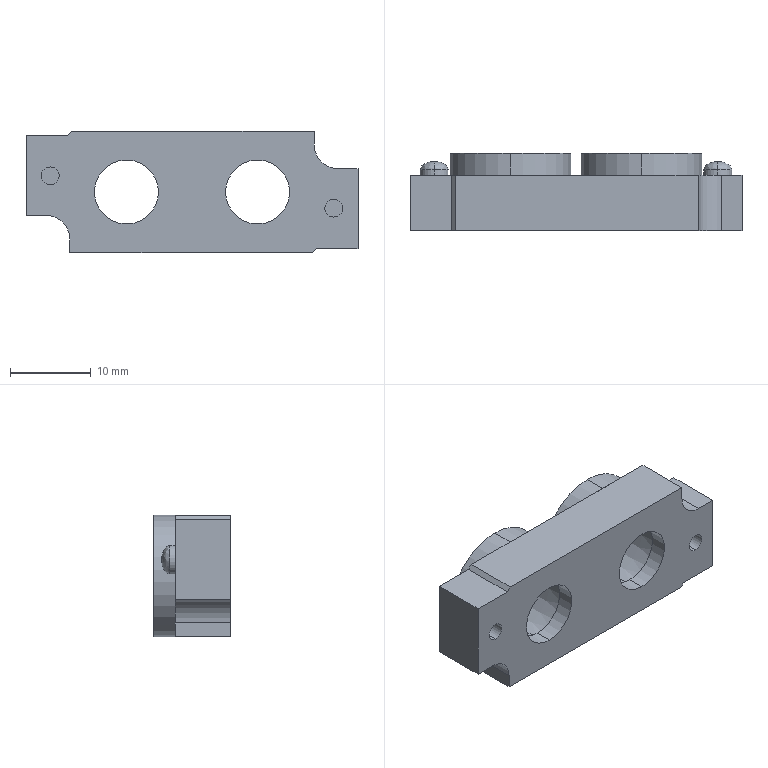Part | STEP file | 11-sy5120-5gz-01_sy5000-6-1-V2.0-V2.011_01 | 1 solid | 48 faces | box 41 x 9.5 x 15 mm | volume 3507 mm3 | plane 22 | cylinder 18 | spline 4 | cone 4 | commonest cylinder face diameters 2.2 x4 3.5 x4 7.9 x4 15 x4 5.8 x2
STEP:
#1=CARTESIAN_POINT('',(-17.5,8.5,2.));
#2=VERTEX_POINT('',#1);
#3=CARTESIAN_POINT('',(-17.5,7.5,3.75));
#4=VERTEX_POINT('',#3);
#5=CARTESIAN_POINT('',(-17.5,8.5,2.));
#6=CARTESIAN_POINT('',(-17.5,8.5,3.025));
#7=CARTESIAN_POINT('',(-17.5,8.086,3.75));
#8=CARTESIAN_POINT('',(-17.5,7.5,3.75));
#9=(BOUNDED_CURVE()B_SPLINE_CURVE(3,(#5,#6,#7,#8),.UNSPECIFIED.,.F.,.F.)B_SPLINE_CURVE_WITH_KNOTS((4,4),(4.712,6.283),.UNSPECIFIED.)CURVE()GEOMETRIC_REPRESENTATION_ITEM()RATIONAL_B_SPLINE_CURVE((1.,0.8047,0.8047,1.))REPRESENTATION_ITEM(''));
#10=EDGE_CURVE('',#2,#4,#9,.T.);
#11=ORIENTED_EDGE('',*,*,#10,.F.);
#12=CARTESIAN_POINT('',(-17.5,7.5,0.25));
#13=VERTEX_POINT('',#12);
#14=CARTESIAN_POINT('',(-17.5,8.5,2.));
#15=CARTESIAN_POINT('',(-17.5,8.5,0.9749));
#16=CARTESIAN_POINT('',(-17.5,8.086,0.25));
#17=CARTESIAN_POINT('',(-17.5,7.5,0.25));
#18=(BOUNDED_CURVE()B_SPLINE_CURVE(3,(#14,#15,#16,#17),.UNSPECIFIED.,.F.,.F.)B_SPLINE_CURVE_WITH_KNOTS((4,4),(4.712,6.283),.UNSPECIFIED.)CURVE()GEOMETRIC_REPRESENTATION_ITEM()RATIONAL_B_SPLINE_CURVE((1.,0.8047,0.8047,1.))REPRESENTATION_ITEM(''));
#19=EDGE_CURVE('',#2,#13,#18,.T.);
#20=ORIENTED_EDGE('',*,*,#19,.T.);
#21=CARTESIAN_POINT('',(-17.5,7.5,2.));
#22=DIRECTION('',(0.,1.,0.));
#23=DIRECTION('',(0.,0.,1.));
#24=AXIS2_PLACEMENT_3D('',#21,#22,#23);
#25=CIRCLE('',#24,1.75);
#26=EDGE_CURVE('',#13,#4,#25,.T.);
#27=ORIENTED_EDGE('',*,*,#26,.T.);
#28=EDGE_LOOP('',(#11,#20,#27));
#29=FACE_OUTER_BOUND('',#28,.T.);
#30=CARTESIAN_POINT('',(-17.5,8.5,2.));
#31=CARTESIAN_POINT('',(-17.5,8.5,2.));
#32=CARTESIAN_POINT('',(-17.5,8.5,2.));
#33=CARTESIAN_POINT('',(-17.5,8.5,2.));
#34=CARTESIAN_POINT('',(-17.5,8.5,0.9749));
#35=CARTESIAN_POINT('',(-19.55,8.5,0.9749));
#36=CARTESIAN_POINT('',(-19.55,8.5,3.025));
#37=CARTESIAN_POINT('',(-17.5,8.5,3.025));
#38=CARTESIAN_POINT('',(-17.5,8.086,0.25));
#39=CARTESIAN_POINT('',(-21.,8.086,0.25));
#40=CARTESIAN_POINT('',(-21.,8.086,3.75));
#41=CARTESIAN_POINT('',(-17.5,8.086,3.75));
#42=CARTESIAN_POINT('',(-17.5,7.5,0.25));
#43=CARTESIAN_POINT('',(-21.,7.5,0.25));
#44=CARTESIAN_POINT('',(-21.,7.5,3.75));
#45=CARTESIAN_POINT('',(-17.5,7.5,3.75));
#46=(BOUNDED_SURFACE()B_SPLINE_SURFACE(3,3,((#30,#31,#32,#33),(#34,#35,#36,#37),(#38,#39,#40,#41),(#42,#43,#44,#45)),.UNSPECIFIED.,.F.,.F.,.F.)B_SPLINE_SURFACE_WITH_KNOTS((4,4),(4,4),(0.,1.),(0.,1.),.UNSPECIFIED.)GEOMETRIC_REPRESENTATION_ITEM()RATIONAL_B_SPLINE_SURFACE(((1.,0.3333,0.3333,1.),(0.8047,0.2682,0.2682,0.8047),(0.8047,0.2682,0.2682,0.8047),(1.,0.3333,0.3333,1.)))REPRESENTATION_ITEM('')SURFACE());
#47=ADVANCED_FACE('',(#29),#46,.T.);
#48=CARTESIAN_POINT('',(17.5,8.5,-2.));
#49=VERTEX_POINT('',#48);
#50=CARTESIAN_POINT('',(17.5,7.5,-0.25));
#51=VERTEX_POINT('',#50);
#52=CARTESIAN_POINT('',(17.5,8.5,-2.));
#53=CARTESIAN_POINT('',(17.5,8.5,-0.9749));
#54=CARTESIAN_POINT('',(17.5,8.086,-0.25));
#55=CARTESIAN_POINT('',(17.5,7.5,-0.25));
#56=(BOUNDED_CURVE()B_SPLINE_CURVE(3,(#52,#53,#54,#55),.UNSPECIFIED.,.F.,.F.)B_SPLINE_CURVE_WITH_KNOTS((4,4),(4.712,6.283),.UNSPECIFIED.)CURVE()GEOMETRIC_REPRESENTATION_ITEM()RATIONAL_B_SPLINE_CURVE((1.,0.8047,0.8047,1.))REPRESENTATION_ITEM(''));
#57=EDGE_CURVE('',#49,#51,#56,.T.);
#58=ORIENTED_EDGE('',*,*,#57,.F.);
#59=CARTESIAN_POINT('',(17.5,7.5,-3.75));
#60=VERTEX_POINT('',#59);
#61=CARTESIAN_POINT('',(17.5,8.5,-2.));
#62=CARTESIAN_POINT('',(17.5,8.5,-3.025));
#63=CARTESIAN_POINT('',(17.5,8.086,-3.75));
#64=CARTESIAN_POINT('',(17.5,7.5,-3.75));
#65=(BOUNDED_CURVE()B_SPLINE_CURVE(3,(#61,#62,#63,#64),.UNSPECIFIED.,.F.,.F.)B_SPLINE_CURVE_WITH_KNOTS((4,4),(4.712,6.283),.UNSPECIFIED.)CURVE()GEOMETRIC_REPRESENTATION_ITEM()RATIONAL_B_SPLINE_CURVE((1.,0.8047,0.8047,1.))REPRESENTATION_ITEM(''));
#66=EDGE_CURVE('',#49,#60,#65,.T.);
#67=ORIENTED_EDGE('',*,*,#66,.T.);
#68=CARTESIAN_POINT('',(17.5,7.5,-2.));
#69=DIRECTION('',(0.,1.,0.));
#70=DIRECTION('',(0.,0.,1.));
#71=AXIS2_PLACEMENT_3D('',#68,#69,#70);
#72=CIRCLE('',#71,1.75);
#73=EDGE_CURVE('',#60,#51,#72,.T.);
#74=ORIENTED_EDGE('',*,*,#73,.T.);
#75=EDGE_LOOP('',(#58,#67,#74));
#76=FACE_OUTER_BOUND('',#75,.T.);
#77=CARTESIAN_POINT('',(17.5,8.5,-2.));
#78=CARTESIAN_POINT('',(17.5,8.5,-2.));
#79=CARTESIAN_POINT('',(17.5,8.5,-2.));
#80=CARTESIAN_POINT('',(17.5,8.5,-2.));
#81=CARTESIAN_POINT('',(17.5,8.5,-3.025));
#82=CARTESIAN_POINT('',(15.45,8.5,-3.025));
#83=CARTESIAN_POINT('',(15.45,8.5,-0.9749));
#84=CARTESIAN_POINT('',(17.5,8.5,-0.9749));
#85=CARTESIAN_POINT('',(17.5,8.086,-3.75));
#86=CARTESIAN_POINT('',(14.,8.086,-3.75));
#87=CARTESIAN_POINT('',(14.,8.086,-0.25));
#88=CARTESIAN_POINT('',(17.5,8.086,-0.25));
#89=CARTESIAN_POINT('',(17.5,7.5,-3.75));
#90=CARTESIAN_POINT('',(14.,7.5,-3.75));
#91=CARTESIAN_POINT('',(14.,7.5,-0.25));
#92=CARTESIAN_POINT('',(17.5,7.5,-0.25));
#93=(BOUNDED_SURFACE()B_SPLINE_SURFACE(3,3,((#77,#78,#79,#80),(#81,#82,#83,#84),(#85,#86,#87,#88),(#89,#90,#91,#92)),.UNSPECIFIED.,.F.,.F.,.F.)B_SPLINE_SURFACE_WITH_KNOTS((4,4),(4,4),(0.,1.),(0.,1.),.UNSPECIFIED.)GEOMETRIC_REPRESENTATION_ITEM()RATIONAL_B_SPLINE_SURFACE(((1.,0.3333,0.3333,1.),(0.8047,0.2682,0.2682,0.8047),(0.8047,0.2682,0.2682,0.8047),(1.,0.3333,0.3333,1.)))REPRESENTATION_ITEM('')SURFACE());
#94=ADVANCED_FACE('',(#76),#93,.T.);
#95=CARTESIAN_POINT('',(-8.1,2.1,-4.633));
#96=VERTEX_POINT('',#95);
#97=CARTESIAN_POINT('',(-8.1,2.1,4.633));
#98=VERTEX_POINT('',#97);
#99=CARTESIAN_POINT('',(-8.1,2.1,0.));
#100=DIRECTION('',(0.,1.,0.));
#101=DIRECTION('',(0.,0.,1.));
#102=AXIS2_PLACEMENT_3D('',#99,#100,#101);
#103=CIRCLE('',#102,4.633);
#104=EDGE_CURVE('',#96,#98,#103,.T.);
#105=ORIENTED_EDGE('',*,*,#104,.F.);
#106=CARTESIAN_POINT('',(-8.1,9.5,-4.864));
#107=VERTEX_POINT('',#106);
#108=CARTESIAN_POINT('',(-8.1,9.5,-4.864));
#109=DIRECTION('',(0.,0.9995,-0.0312));
#110=VECTOR('',#109,1000.);
#111=LINE('',#108,#110);
#112=EDGE_CURVE('',#96,#107,#111,.T.);
#113=ORIENTED_EDGE('',*,*,#112,.T.);
#114=CARTESIAN_POINT('',(-8.1,9.5,4.864));
#115=VERTEX_POINT('',#114);
#116=CARTESIAN_POINT('',(-8.1,9.5,0.));
#117=DIRECTION('',(0.,1.,0.));
#118=DIRECTION('',(0.,0.,1.));
#119=AXIS2_PLACEMENT_3D('',#116,#117,#118);
#120=CIRCLE('',#119,4.864);
#121=EDGE_CURVE('',#107,#115,#120,.T.);
#122=ORIENTED_EDGE('',*,*,#121,.T.);
#123=CARTESIAN_POINT('',(-8.1,9.5,4.864));
#124=DIRECTION('',(0.,0.9995,0.0312));
#125=VECTOR('',#124,1000.);
#126=LINE('',#123,#125);
#127=EDGE_CURVE('',#98,#115,#126,.T.);
#128=ORIENTED_EDGE('',*,*,#127,.F.);
#129=EDGE_LOOP('',(#105,#113,#122,#128));
#130=FACE_OUTER_BOUND('',#129,.T.);
#131=CARTESIAN_POINT('',(-8.1,9.5,0.));
#132=DIRECTION('',(0.,1.,0.));
#133=DIRECTION('',(0.,0.,1.));
#134=AXIS2_PLACEMENT_3D('',#131,#132,#133);
#135=CONICAL_SURFACE('',#134,4.864,0.03121);
#136=ADVANCED_FACE('',(#130),#135,.F.);
#137=CARTESIAN_POINT('',(-8.1,0.,-3.95));
#138=VERTEX_POINT('',#137);
#139=CARTESIAN_POINT('',(-8.1,0.,3.95));
#140=VERTEX_POINT('',#139);
#141=CARTESIAN_POINT('',(-8.1,0.,0.));
#142=DIRECTION('',(0.,1.,0.));
#143=DIRECTION('',(0.,0.,1.));
#144=AXIS2_PLACEMENT_3D('',#141,#142,#143);
#145=CIRCLE('',#144,3.95);
#146=EDGE_CURVE('',#138,#140,#145,.T.);
#147=ORIENTED_EDGE('',*,*,#146,.F.);
#148=CARTESIAN_POINT('',(-8.1,2.1,-3.95));
#149=VERTEX_POINT('',#148);
#150=CARTESIAN_POINT('',(-8.1,9.5,-3.95));
#151=DIRECTION('',(0.,1.,0.));
#152=VECTOR('',#151,1000.);
#153=LINE('',#150,#152);
#154=EDGE_CURVE('',#138,#149,#153,.T.);
#155=ORIENTED_EDGE('',*,*,#154,.T.);
#156=CARTESIAN_POINT('',(-8.1,2.1,3.95));
#157=VERTEX_POINT('',#156);
#158=CARTESIAN_POINT('',(-8.1,2.1,0.));
#159=DIRECTION('',(0.,1.,0.));
#160=DIRECTION('',(0.,0.,1.));
#161=AXIS2_PLACEMENT_3D('',#158,#159,#160);
#162=CIRCLE('',#161,3.95);
#163=EDGE_CURVE('',#149,#157,#162,.T.);
#164=ORIENTED_EDGE('',*,*,#163,.T.);
#165=CARTESIAN_POINT('',(-8.1,9.5,3.95));
#166=DIRECTION('',(0.,1.,0.));
#167=VECTOR('',#166,1000.);
#168=LINE('',#165,#167);
#169=EDGE_CURVE('',#140,#157,#168,.T.);
#170=ORIENTED_EDGE('',*,*,#169,.F.);
#171=EDGE_LOOP('',(#147,#155,#164,#170));
#172=FACE_OUTER_BOUND('',#171,.T.);
#173=CARTESIAN_POINT('',(-8.1,9.5,0.));
#174=DIRECTION('',(0.,1.,0.));
#175=DIRECTION('',(0.,0.,1.));
#176=AXIS2_PLACEMENT_3D('',#173,#174,#175);
#177=CYLINDRICAL_SURFACE('',#176,3.95);
#178=ADVANCED_FACE('',(#172),#177,.F.);
#179=CARTESIAN_POINT('',(8.1,2.1,-4.633));
#180=VERTEX_POINT('',#179);
#181=CARTESIAN_POINT('',(8.1,2.1,4.633));
#182=VERTEX_POINT('',#181);
#183=CARTESIAN_POINT('',(8.1,2.1,0.));
#184=DIRECTION('',(0.,1.,0.));
#185=DIRECTION('',(0.,0.,1.));
#186=AXIS2_PLACEMENT_3D('',#183,#184,#185);
#187=CIRCLE('',#186,4.633);
#188=EDGE_CURVE('',#180,#182,#187,.T.);
#189=ORIENTED_EDGE('',*,*,#188,.F.);
#190=CARTESIAN_POINT('',(8.1,9.5,-4.864));
#191=VERTEX_POINT('',#190);
#192=CARTESIAN_POINT('',(8.1,9.5,-4.864));
#193=DIRECTION('',(0.,0.9995,-0.0312));
#194=VECTOR('',#193,1000.);
#195=LINE('',#192,#194);
#196=EDGE_CURVE('',#180,#191,#195,.T.);
#197=ORIENTED_EDGE('',*,*,#196,.T.);
#198=CARTESIAN_POINT('',(8.1,9.5,4.864));
#199=VERTEX_POINT('',#198);
#200=CARTESIAN_POINT('',(8.1,9.5,0.));
#201=DIRECTION('',(0.,1.,0.));
#202=DIRECTION('',(0.,0.,1.));
#203=AXIS2_PLACEMENT_3D('',#200,#201,#202);
#204=CIRCLE('',#203,4.864);
#205=EDGE_CURVE('',#191,#199,#204,.T.);
#206=ORIENTED_EDGE('',*,*,#205,.T.);
#207=CARTESIAN_POINT('',(8.1,9.5,4.864));
#208=DIRECTION('',(0.,0.9995,0.0312));
#209=VECTOR('',#208,1000.);
#210=LINE('',#207,#209);
#211=EDGE_CURVE('',#182,#199,#210,.T.);
#212=ORIENTED_EDGE('',*,*,#211,.F.);
#213=EDGE_LOOP('',(#189,#197,#206,#212));
#214=FACE_OUTER_BOUND('',#213,.T.);
#215=CARTESIAN_POINT('',(8.1,9.5,0.));
#216=DIRECTION('',(0.,1.,0.));
#217=DIRECTION('',(0.,0.,1.));
#218=AXIS2_PLACEMENT_3D('',#215,#216,#217);
#219=CONICAL_SURFACE('',#218,4.864,0.03121);
#220=ADVANCED_FACE('',(#214),#219,.F.);
#221=CARTESIAN_POINT('',(8.1,0.,-3.95));
#222=VERTEX_POINT('',#221);
#223=CARTESIAN_POINT('',(8.1,0.,3.95));
#224=VERTEX_POINT('',#223);
#225=CARTESIAN_POINT('',(8.1,0.,0.));
#226=DIRECTION('',(0.,1.,0.));
#227=DIRECTION('',(0.,0.,1.));
#228=AXIS2_PLACEMENT_3D('',#225,#226,#227);
#229=CIRCLE('',#228,3.95);
#230=EDGE_CURVE('',#222,#224,#229,.T.);
#231=ORIENTED_EDGE('',*,*,#230,.F.);
#232=CARTESIAN_POINT('',(8.1,2.1,-3.95));
#233=VERTEX_POINT('',#232);
#234=CARTESIAN_POINT('',(8.1,9.5,-3.95));
#235=DIRECTION('',(0.,1.,0.));
#236=VECTOR('',#235,1000.);
#237=LINE('',#234,#236);
#238=EDGE_CURVE('',#222,#233,#237,.T.);
#239=ORIENTED_EDGE('',*,*,#238,.T.);
#240=CARTESIAN_POINT('',(8.1,2.1,3.95));
#241=VERTEX_POINT('',#240);
#242=CARTESIAN_POINT('',(8.1,2.1,0.));
#243=DIRECTION('',(0.,1.,0.));
#244=DIRECTION('',(0.,0.,1.));
#245=AXIS2_PLACEMENT_3D('',#242,#243,#244);
#246=CIRCLE('',#245,3.95);
#247=EDGE_CURVE('',#233,#241,#246,.T.);
#248=ORIENTED_EDGE('',*,*,#247,.T.);
#249=CARTESIAN_POINT('',(8.1,9.5,3.95));
#250=DIRECTION('',(0.,1.,0.));
#251=VECTOR('',#250,1000.);
#252=LINE('',#249,#251);
#253=EDGE_CURVE('',#224,#241,#252,.T.);
#254=ORIENTED_EDGE('',*,*,#253,.F.);
#255=EDGE_LOOP('',(#231,#239,#248,#254));
#256=FACE_OUTER_BOUND('',#255,.T.);
#257=CARTESIAN_POINT('',(8.1,9.5,0.));
#258=DIRECTION('',(0.,1.,0.));
#259=DIRECTION('',(0.,0.,1.));
#260=AXIS2_PLACEMENT_3D('',#257,#258,#259);
#261=CYLINDRICAL_SURFACE('',#260,3.95);
#262=ADVANCED_FACE('',(#256),#261,.F.);
#263=CARTESIAN_POINT('',(-17.5,7.5,2.));
#264=DIRECTION('',(0.,1.,0.));
#265=DIRECTION('',(0.,0.,1.));
#266=AXIS2_PLACEMENT_3D('',#263,#264,#265);
#267=CIRCLE('',#266,1.75);
#268=EDGE_CURVE('',#4,#13,#267,.T.);
#269=ORIENTED_EDGE('',*,*,#268,.F.);
#270=CARTESIAN_POINT('',(-17.5,6.8,3.75));
#271=VERTEX_POINT('',#270);
#272=CARTESIAN_POINT('',(-17.5,7.5,3.75));
#273=DIRECTION('',(0.,-1.,0.));
#274=VECTOR('',#273,1000.);
#275=LINE('',#272,#274);
#276=EDGE_CURVE('',#4,#271,#275,.T.);
#277=ORIENTED_EDGE('',*,*,#276,.T.);
#278=CARTESIAN_POINT('',(-17.5,6.8,0.25));
#279=VERTEX_POINT('',#278);
#280=CARTESIAN_POINT('',(-17.5,6.8,2.));
#281=DIRECTION('',(0.,1.,0.));
#282=DIRECTION('',(0.,0.,1.));
#283=AXIS2_PLACEMENT_3D('',#280,#281,#282);
#284=CIRCLE('',#283,1.75);
#285=EDGE_CURVE('',#271,#279,#284,.T.);
#286=ORIENTED_EDGE('',*,*,#285,.T.);
#287=CARTESIAN_POINT('',(-17.5,7.5,0.25));
#288=DIRECTION('',(0.,-1.,0.));
#289=VECTOR('',#288,1000.);
#290=LINE('',#287,#289);
#291=EDGE_CURVE('',#13,#279,#290,.T.);
#292=ORIENTED_EDGE('',*,*,#291,.F.);
#293=EDGE_LOOP('',(#269,#277,#286,#292));
#294=FACE_OUTER_BOUND('',#293,.T.);
#295=CARTESIAN_POINT('',(-17.5,7.5,2.));
#296=DIRECTION('',(0.,-1.,0.));
#297=DIRECTION('',(0.,0.,-1.));
#298=AXIS2_PLACEMENT_3D('',#295,#296,#297);
#299=CYLINDRICAL_SURFACE('',#298,1.75);
#300=ADVANCED_FACE('',(#294),#299,.T.);
#301=CARTESIAN_POINT('',(17.5,7.5,-2.));
#302=DIRECTION('',(0.,1.,0.));
#303=DIRECTION('',(0.,0.,1.));
#304=AXIS2_PLACEMENT_3D('',#301,#302,#303);
#305=CIRCLE('',#304,1.75);
#306=EDGE_CURVE('',#51,#60,#305,.T.);
#307=ORIENTED_EDGE('',*,*,#306,.F.);
#308=CARTESIAN_POINT('',(17.5,6.8,-0.25));
#309=VERTEX_POINT('',#308);
#310=CARTESIAN_POINT('',(17.5,7.5,-0.25));
#311=DIRECTION('',(0.,-1.,0.));
#312=VECTOR('',#311,1000.);
#313=LINE('',#310,#312);
#314=EDGE_CURVE('',#51,#309,#313,.T.);
#315=ORIENTED_EDGE('',*,*,#314,.T.);
#316=CARTESIAN_POINT('',(17.5,6.8,-3.75));
#317=VERTEX_POINT('',#316);
#318=CARTESIAN_POINT('',(17.5,6.8,-2.));
#319=DIRECTION('',(0.,1.,0.));
#320=DIRECTION('',(0.,0.,1.));
#321=AXIS2_PLACEMENT_3D('',#318,#319,#320);
#322=CIRCLE('',#321,1.75);
#323=EDGE_CURVE('',#309,#317,#322,.T.);
#324=ORIENTED_EDGE('',*,*,#323,.T.);
#325=CARTESIAN_POINT('',(17.5,7.5,-3.75));
#326=DIRECTION('',(0.,-1.,0.));
#327=VECTOR('',#326,1000.);
#328=LINE('',#325,#327);
#329=EDGE_CURVE('',#60,#317,#328,.T.);
#330=ORIENTED_EDGE('',*,*,#329,.F.);
#331=EDGE_LOOP('',(#307,#315,#324,#330));
#332=FACE_OUTER_BOUND('',#331,.T.);
#333=CARTESIAN_POINT('',(17.5,7.5,-2.));
#334=DIRECTION('',(0.,-1.,0.));
#335=DIRECTION('',(0.,0.,-1.));
#336=AXIS2_PLACEMENT_3D('',#333,#334,#335);
#337=CYLINDRICAL_SURFACE('',#336,1.75);
#338=ADVANCED_FACE('',(#332),#337,.T.);
#339=CARTESIAN_POINT('',(-8.1,9.5,7.5));
#340=VERTEX_POINT('',#339);
#341=CARTESIAN_POINT('',(-8.1,9.5,-7.5));
#342=VERTEX_POINT('',#341);
#343=CARTESIAN_POINT('',(-8.1,9.5,0.));
#344=DIRECTION('',(0.,1.,0.));
#345=DIRECTION('',(0.,0.,1.));
#346=AXIS2_PLACEMENT_3D('',#343,#344,#345);
#347=CIRCLE('',#346,7.5);
#348=EDGE_CURVE('',#340,#342,#347,.T.);
#349=ORIENTED_EDGE('',*,*,#348,.F.);
#350=CARTESIAN_POINT('',(-8.1,6.8,7.5));
#351=VERTEX_POINT('',#350);
#352=CARTESIAN_POINT('',(-8.1,9.5,7.5));
#353=DIRECTION('',(0.,-1.,0.));
#354=VECTOR('',#353,1000.);
#355=LINE('',#352,#354);
#356=EDGE_CURVE('',#340,#351,#355,.T.);
#357=ORIENTED_EDGE('',*,*,#356,.T.);
#358=CARTESIAN_POINT('',(-8.1,6.8,-7.5));
#359=VERTEX_POINT('',#358);
#360=CARTESIAN_POINT('',(-8.1,6.8,0.));
#361=DIRECTION('',(0.,1.,0.));
#362=DIRECTION('',(0.,0.,1.));
#363=AXIS2_PLACEMENT_3D('',#360,#361,#362);
#364=CIRCLE('',#363,7.5);
#365=EDGE_CURVE('',#351,#359,#364,.T.);
#366=ORIENTED_EDGE('',*,*,#365,.T.);
#367=CARTESIAN_POINT('',(-8.1,9.5,-7.5));
#368=DIRECTION('',(0.,-1.,0.));
#369=VECTOR('',#368,1000.);
#370=LINE('',#367,#369);
#371=EDGE_CURVE('',#342,#359,#370,.T.);
#372=ORIENTED_EDGE('',*,*,#371,.F.);
#373=EDGE_LOOP('',(#349,#357,#366,#372));
#374=FACE_OUTER_BOUND('',#373,.T.);
#375=CARTESIAN_POINT('',(-8.1,9.5,0.));
#376=DIRECTION('',(0.,-1.,0.));
#377=DIRECTION('',(0.,0.,-1.));
#378=AXIS2_PLACEMENT_3D('',#375,#376,#377);
#379=CYLINDRICAL_SURFACE('',#378,7.5);
#380=ADVANCED_FACE('',(#374),#379,.T.);
#381=CARTESIAN_POINT('',(8.1,9.5,7.5));
#382=VERTEX_POINT('',#381);
#383=CARTESIAN_POINT('',(8.1,9.5,-7.5));
#384=VERTEX_POINT('',#383);
#385=CARTESIAN_POINT('',(8.1,9.5,0.));
#386=DIRECTION('',(0.,1.,0.));
#387=DIRECTION('',(0.,0.,1.));
#388=AXIS2_PLACEMENT_3D('',#385,#386,#387);
#389=CIRCLE('',#388,7.5);
#390=EDGE_CURVE('',#382,#384,#389,.T.);
#391=ORIENTED_EDGE('',*,*,#390,.F.);
#392=CARTESIAN_POINT('',(8.1,6.8,7.5));
#393=VERTEX_POINT('',#392);
#394=CARTESIAN_POINT('',(8.1,9.5,7.5));
#395=DIRECTION('',(0.,-1.,0.));
#396=VECTOR('',#395,1000.);
#397=LINE('',#394,#396);
#398=EDGE_CURVE('',#382,#393,#397,.T.);
#399=ORIENTED_EDGE('',*,*,#398,.T.);
#400=CARTESIAN_POINT('',(8.1,6.8,-7.5));
#401=VERTEX_POINT('',#400);
#402=CARTESIAN_POINT('',(8.1,6.8,0.));
#403=DIRECTION('',(0.,1.,0.));
#404=DIRECTION('',(0.,0.,1.));
#405=AXIS2_PLACEMENT_3D('',#402,#403,#404);
#406=CIRCLE('',#405,7.5);
#407=EDGE_CURVE('',#393,#401,#406,.T.);
#408=ORIENTED_EDGE('',*,*,#407,.T.);
#409=CARTESIAN_POINT('',(8.1,9.5,-7.5));
#410=DIRECTION('',(0.,-1.,0.));
#411=VECTOR('',#410,1000.);
#412=LINE('',#409,#411);
#413=EDGE_CURVE('',#384,#401,#412,.T.);
#414=ORIENTED_EDGE('',*,*,#413,.F.);
#415=EDGE_LOOP('',(#391,#399,#408,#414));
#416=FACE_OUTER_BOUND('',#415,.T.);
#417=CARTESIAN_POINT('',(8.1,9.5,0.));
#418=DIRECTION('',(0.,-1.,0.));
#419=DIRECTION('',(0.,0.,-1.));
#420=AXIS2_PLACEMENT_3D('',#417,#418,#419);
#421=CYLINDRICAL_SURFACE('',#420,7.5);
#422=ADVANCED_FACE('',(#416),#421,.T.);
#423=CARTESIAN_POINT('',(17.5,6.8,-3.1));
#424=VERTEX_POINT('',#423);
#425=CARTESIAN_POINT('',(17.5,6.8,-0.9));
#426=VERTEX_POINT('',#425);
#427=CARTESIAN_POINT('',(17.5,6.8,-2.));
#428=DIRECTION('',(0.,1.,0.));
#429=DIRECTION('',(0.,0.,1.));
#430=AXIS2_PLACEMENT_3D('',#427,#428,#429);
#431=CIRCLE('',#430,1.1);
#432=EDGE_CURVE('',#424,#426,#431,.T.);
#433=ORIENTED_EDGE('',*,*,#432,.T.);
#434=CARTESIAN_POINT('',(17.5,0.,-0.9));
#435=VERTEX_POINT('',#434);
#436=CARTESIAN_POINT('',(17.5,6.8,-0.9));
#437=DIRECTION('',(0.,-1.,0.));
#438=VECTOR('',#437,1000.);
#439=LINE('',#436,#438);
#440=EDGE_CURVE('',#426,#435,#439,.T.);
#441=ORIENTED_EDGE('',*,*,#440,.T.);
#442=CARTESIAN_POINT('',(17.5,0.,-3.1));
#443=VERTEX_POINT('',#442);
#444=CARTESIAN_POINT('',(17.5,0.,-2.));
#445=DIRECTION('',(0.,1.,0.));
#446=DIRECTION('',(0.,0.,1.));
#447=AXIS2_PLACEMENT_3D('',#444,#445,#446);
#448=CIRCLE('',#447,1.1);
#449=EDGE_CURVE('',#443,#435,#448,.T.);
#450=ORIENTED_EDGE('',*,*,#449,.F.);
#451=CARTESIAN_POINT('',(17.5,6.8,-3.1));
#452=DIRECTION('',(0.,-1.,0.));
#453=VECTOR('',#452,1000.);
#454=LINE('',#451,#453);
#455=EDGE_CURVE('',#424,#443,#454,.T.);
#456=ORIENTED_EDGE('',*,*,#455,.F.);
#457=EDGE_LOOP('',(#433,#441,#450,#456));
#458=FACE_OUTER_BOUND('',#457,.T.);
#459=CARTESIAN_POINT('',(17.5,6.8,-2.));
#460=DIRECTION('',(0.,-1.,0.));
#461=DIRECTION('',(0.,0.,-1.));
#462=AXIS2_PLACEMENT_3D('',#459,#460,#461);
#463=CYLINDRICAL_SURFACE('',#462,1.1);
#464=ADVANCED_FACE('',(#458),#463,.F.);
#465=CARTESIAN_POINT('',(-17.5,6.8,0.9));
#466=VERTEX_POINT('',#465);
#467=CARTESIAN_POINT('',(-17.5,6.8,3.1));
#468=VERTEX_POINT('',#467);
#469=CARTESIAN_POINT('',(-17.5,6.8,2.));
#470=DIRECTION('',(0.,1.,0.));
#471=DIRECTION('',(0.,0.,1.));
#472=AXIS2_PLACEMENT_3D('',#469,#470,#471);
#473=CIRCLE('',#472,1.1);
#474=EDGE_CURVE('',#466,#468,#473,.T.);
#475=ORIENTED_EDGE('',*,*,#474,.T.);
#476=CARTESIAN_POINT('',(-17.5,0.,3.1));
#477=VERTEX_POINT('',#476);
#478=CARTESIAN_POINT('',(-17.5,6.8,3.1));
#479=DIRECTION('',(0.,-1.,0.));
#480=VECTOR('',#479,1000.);
#481=LINE('',#478,#480);
#482=EDGE_CURVE('',#468,#477,#481,.T.);
#483=ORIENTED_EDGE('',*,*,#482,.T.);
#484=CARTESIAN_POINT('',(-17.5,0.,0.9));
#485=VERTEX_POINT('',#484);
#486=CARTESIAN_POINT('',(-17.5,0.,2.));
#487=DIRECTION('',(0.,1.,0.));
#488=DIRECTION('',(0.,0.,1.));
#489=AXIS2_PLACEMENT_3D('',#486,#487,#488);
#490=CIRCLE('',#489,1.1);
#491=EDGE_CURVE('',#485,#477,#490,.T.);
#492=ORIENTED_EDGE('',*,*,#491,.F.);
#493=CARTESIAN_POINT('',(-17.5,6.8,0.9));
#494=DIRECTION('',(0.,-1.,0.));
#495=VECTOR('',#494,1000.);
#496=LINE('',#493,#495);
#497=EDGE_CURVE('',#466,#485,#496,.T.);
#498=ORIENTED_EDGE('',*,*,#497,.F.);
#499=EDGE_LOOP('',(#475,#483,#492,#498));
#500=FACE_OUTER_BOUND('',#499,.T.);
#501=CARTESIAN_POINT('',(-17.5,6.8,2.));
#502=DIRECTION('',(0.,-1.,0.));
#503=DIRECTION('',(0.,0.,-1.));
#504=AXIS2_PLACEMENT_3D('',#501,#502,#503);
#505=CYLINDRICAL_SURFACE('',#504,1.1);
#506=ADVANCED_FACE('',(#500),#505,.F.);
#507=CARTESIAN_POINT('',(-14.9,6.8,7.5));
#508=VERTEX_POINT('',#507);
#509=CARTESIAN_POINT('',(-14.9,6.8,7.5));
#510=DIRECTION('',(1.,0.,0.));
#511=VECTOR('',#510,1000.);
#512=LINE('',#509,#511);
#513=EDGE_CURVE('',#508,#351,#512,.T.);
#514=ORIENTED_EDGE('',*,*,#513,.T.);
#515=CARTESIAN_POINT('',(-8.1,6.8,0.));
#516=DIRECTION('',(0.,1.,0.));
#517=DIRECTION('',(0.,0.,1.));
#518=AXIS2_PLACEMENT_3D('',#515,#516,#517);
#519=CIRCLE('',#518,7.5);
#520=EDGE_CURVE('',#359,#351,#519,.T.);
#521=ORIENTED_EDGE('',*,*,#520,.F.);
#522=CARTESIAN_POINT('',(-15.1,6.8,-7.5));
#523=VERTEX_POINT('',#522);
#524=CARTESIAN_POINT('',(-15.1,6.8,-7.5));
#525=DIRECTION('',(-1.,0.,0.));
#526=VECTOR('',#525,1000.);
#527=LINE('',#524,#526);
#528=EDGE_CURVE('',#359,#523,#527,.T.);
#529=ORIENTED_EDGE('',*,*,#528,.T.);
#530=CARTESIAN_POINT('',(-15.1,6.8,-5.8));
#531=VERTEX_POINT('',#530);
#532=CARTESIAN_POINT('',(-15.1,6.8,-7.5));
#533=DIRECTION('',(0.,0.,1.));
#534=VECTOR('',#533,1000.);
#535=LINE('',#532,#534);
#536=EDGE_CURVE('',#523,#531,#535,.T.);
#537=ORIENTED_EDGE('',*,*,#536,.T.);
#538=CARTESIAN_POINT('',(-18.,6.8,-2.9));
#539=VERTEX_POINT('',#538);
#540=CARTESIAN_POINT('',(-18.,6.8,-5.8));
#541=DIRECTION('',(0.,-1.,0.));
#542=DIRECTION('',(0.,0.,1.));
#543=AXIS2_PLACEMENT_3D('',#540,#541,#542);
#544=CIRCLE('',#543,2.9);
#545=EDGE_CURVE('',#531,#539,#544,.T.);
#546=ORIENTED_EDGE('',*,*,#545,.T.);
#547=CARTESIAN_POINT('',(-20.5,6.8,-2.9));
#548=VERTEX_POINT('',#547);
#549=CARTESIAN_POINT('',(-20.5,6.8,-2.9));
#550=DIRECTION('',(-1.,0.,0.));
#551=VECTOR('',#550,1000.);
#552=LINE('',#549,#551);
#553=EDGE_CURVE('',#539,#548,#552,.T.);
#554=ORIENTED_EDGE('',*,*,#553,.T.);
#555=CARTESIAN_POINT('',(-20.5,6.8,7.));
#556=VERTEX_POINT('',#555);
#557=CARTESIAN_POINT('',(-20.5,6.8,-2.9));
#558=DIRECTION('',(0.,0.,1.));
#559=VECTOR('',#558,1000.);
#560=LINE('',#557,#559);
#561=EDGE_CURVE('',#548,#556,#560,.T.);
#562=ORIENTED_EDGE('',*,*,#561,.T.);
#563=CARTESIAN_POINT('',(-15.4,6.8,7.));
#564=VERTEX_POINT('',#563);
#565=CARTESIAN_POINT('',(-20.5,6.8,7.));
#566=DIRECTION('',(1.,0.,0.));
#567=VECTOR('',#566,1000.);
#568=LINE('',#565,#567);
#569=EDGE_CURVE('',#556,#564,#568,.T.);
#570=ORIENTED_EDGE('',*,*,#569,.T.);
#571=CARTESIAN_POINT('',(-14.9,6.8,7.5));
#572=DIRECTION('',(0.7071,0.,0.7071));
#573=VECTOR('',#572,1000.);
#574=LINE('',#571,#573);
#575=EDGE_CURVE('',#564,#508,#574,.T.);
#576=ORIENTED_EDGE('',*,*,#575,.T.);
#577=EDGE_LOOP('',(#514,#521,#529,#537,#546,#554,#562,#570,#576));
#578=FACE_OUTER_BOUND('',#577,.T.);
#579=CARTESIAN_POINT('',(-17.5,6.8,2.));
#580=DIRECTION('',(0.,1.,0.));
#581=DIRECTION('',(0.,0.,1.));
#582=AXIS2_PLACEMENT_3D('',#579,#580,#581);
#583=CIRCLE('',#582,1.75);
#584=EDGE_CURVE('',#279,#271,#583,.T.);
#585=ORIENTED_EDGE('',*,*,#584,.F.);
#586=ORIENTED_EDGE('',*,*,#285,.F.);
#587=EDGE_LOOP('',(#585,#586));
#588=FACE_BOUND('',#587,.T.);
#589=CARTESIAN_POINT('',(-18.,6.8,-5.8));
#590=DIRECTION('',(0.,1.,0.));
#591=DIRECTION('',(0.,0.,1.));
#592=AXIS2_PLACEMENT_3D('',#589,#590,#591);
#593=PLANE('',#592);
#594=ADVANCED_FACE('',(#578,#588),#593,.T.);
#595=ORIENTED_EDGE('',*,*,#407,.F.);
#596=CARTESIAN_POINT('',(15.1,6.8,7.5));
#597=VERTEX_POINT('',#596);
#598=CARTESIAN_POINT('',(-14.9,6.8,7.5));
#599=DIRECTION('',(1.,0.,0.));
#600=VECTOR('',#599,1000.);
#601=LINE('',#598,#600);
#602=EDGE_CURVE('',#393,#597,#601,.T.);
#603=ORIENTED_EDGE('',*,*,#602,.T.);
#604=CARTESIAN_POINT('',(15.1,6.8,5.8));
#605=VERTEX_POINT('',#604);
#606=CARTESIAN_POINT('',(15.1,6.8,5.8));
#607=DIRECTION('',(0.,0.,-1.));
#608=VECTOR('',#607,1000.);
#609=LINE('',#606,#608);
#610=EDGE_CURVE('',#597,#605,#609,.T.);
#611=ORIENTED_EDGE('',*,*,#610,.T.);
#612=CARTESIAN_POINT('',(18.,6.8,2.9));
#613=VERTEX_POINT('',#612);
#614=CARTESIAN_POINT('',(18.,6.8,5.8));
#615=DIRECTION('',(0.,-1.,0.));
#616=DIRECTION('',(0.,0.,-1.));
#617=AXIS2_PLACEMENT_3D('',#614,#615,#616);
#618=CIRCLE('',#617,2.9);
#619=EDGE_CURVE('',#605,#613,#618,.T.);
#620=ORIENTED_EDGE('',*,*,#619,.T.);
#621=CARTESIAN_POINT('',(20.5,6.8,2.9));
#622=VERTEX_POINT('',#621);
#623=CARTESIAN_POINT('',(18.,6.8,2.9));
#624=DIRECTION('',(1.,0.,0.));
#625=VECTOR('',#624,1000.);
#626=LINE('',#623,#625);
#627=EDGE_CURVE('',#613,#622,#626,.T.);
#628=ORIENTED_EDGE('',*,*,#627,.T.);
#629=CARTESIAN_POINT('',(20.5,6.8,-7.));
#630=VERTEX_POINT('',#629);
#631=CARTESIAN_POINT('',(20.5,6.8,-7.));
#632=DIRECTION('',(0.,0.,-1.));
#633=VECTOR('',#632,1000.);
#634=LINE('',#631,#633);
#635=EDGE_CURVE('',#622,#630,#634,.T.);
#636=ORIENTED_EDGE('',*,*,#635,.T.);
#637=CARTESIAN_POINT('',(15.4,6.8,-7.));
#638=VERTEX_POINT('',#637);
#639=CARTESIAN_POINT('',(15.4,6.8,-7.));
#640=DIRECTION('',(-1.,0.,0.));
#641=VECTOR('',#640,1000.);
#642=LINE('',#639,#641);
#643=EDGE_CURVE('',#630,#638,#642,.T.);
#644=ORIENTED_EDGE('',*,*,#643,.T.);
#645=CARTESIAN_POINT('',(14.9,6.8,-7.5));
#646=VERTEX_POINT('',#645);
#647=CARTESIAN_POINT('',(14.9,6.8,-7.5));
#648=DIRECTION('',(-0.7071,0.,-0.7071));
#649=VECTOR('',#648,1000.);
#650=LINE('',#647,#649);
#651=EDGE_CURVE('',#638,#646,#650,.T.);
#652=ORIENTED_EDGE('',*,*,#651,.T.);
#653=CARTESIAN_POINT('',(-15.1,6.8,-7.5));
#654=DIRECTION('',(-1.,0.,0.));
#655=VECTOR('',#654,1000.);
#656=LINE('',#653,#655);
#657=EDGE_CURVE('',#646,#401,#656,.T.);
#658=ORIENTED_EDGE('',*,*,#657,.T.);
#659=EDGE_LOOP('',(#595,#603,#611,#620,#628,#636,#644,#652,#658));
#660=FACE_OUTER_BOUND('',#659,.T.);
#661=CARTESIAN_POINT('',(17.5,6.8,-2.));
#662=DIRECTION('',(0.,1.,0.));
#663=DIRECTION('',(0.,0.,1.));
#664=AXIS2_PLACEMENT_3D('',#661,#662,#663);
#665=CIRCLE('',#664,1.75);
#666=EDGE_CURVE('',#317,#309,#665,.T.);
#667=ORIENTED_EDGE('',*,*,#666,.F.);
#668=ORIENTED_EDGE('',*,*,#323,.F.);
#669=EDGE_LOOP('',(#667,#668));
#670=FACE_BOUND('',#669,.T.);
#671=CARTESIAN_POINT('',(-18.,6.8,-5.8));
#672=DIRECTION('',(0.,1.,0.));
#673=DIRECTION('',(0.,0.,1.));
#674=AXIS2_PLACEMENT_3D('',#671,#672,#673);
#675=PLANE('',#674);
#676=ADVANCED_FACE('',(#660,#670),#675,.T.);
#677=CARTESIAN_POINT('',(-15.1,6.8,-7.5));
#678=DIRECTION('',(-1.,0.,0.));
#679=VECTOR('',#678,1000.);
#680=LINE('',#677,#679);
#681=EDGE_CURVE('',#401,#359,#680,.T.);
#682=ORIENTED_EDGE('',*,*,#681,.T.);
#683=ORIENTED_EDGE('',*,*,#365,.F.);
#684=CARTESIAN_POINT('',(-14.9,6.8,7.5));
#685=DIRECTION('',(1.,0.,0.));
#686=VECTOR('',#685,1000.);
#687=LINE('',#684,#686);
#688=EDGE_CURVE('',#351,#393,#687,.T.);
#689=ORIENTED_EDGE('',*,*,#688,.T.);
#690=CARTESIAN_POINT('',(8.1,6.8,0.));
#691=DIRECTION('',(0.,1.,0.));
#692=DIRECTION('',(0.,0.,1.));
#693=AXIS2_PLACEMENT_3D('',#690,#691,#692);
#694=CIRCLE('',#693,7.5);
#695=EDGE_CURVE('',#401,#393,#694,.T.);
#696=ORIENTED_EDGE('',*,*,#695,.F.);
#697=EDGE_LOOP('',(#682,#683,#689,#696));
#698=FACE_OUTER_BOUND('',#697,.T.);
#699=CARTESIAN_POINT('',(-18.,6.8,-5.8));
#700=DIRECTION('',(0.,1.,0.));
#701=DIRECTION('',(0.,0.,1.));
#702=AXIS2_PLACEMENT_3D('',#699,#700,#701);
#703=PLANE('',#702);
#704=ADVANCED_FACE('',(#698),#703,.T.);
#705=CARTESIAN_POINT('',(-8.1,0.,0.));
#706=DIRECTION('',(0.,1.,0.));
#707=DIRECTION('',(0.,0.,1.));
#708=AXIS2_PLACEMENT_3D('',#705,#706,#707);
#709=CIRCLE('',#708,3.95);
#710=EDGE_CURVE('',#140,#138,#709,.T.);
#711=ORIENTED_EDGE('',*,*,#710,.T.);
#712=ORIENTED_EDGE('',*,*,#146,.T.);
#713=EDGE_LOOP('',(#711,#712));
#714=FACE_BOUND('',#713,.T.);
#715=CARTESIAN_POINT('',(8.1,0.,0.));
#716=DIRECTION('',(0.,1.,0.));
#717=DIRECTION('',(0.,0.,1.));
#718=AXIS2_PLACEMENT_3D('',#715,#716,#717);
#719=CIRCLE('',#718,3.95);
#720=EDGE_CURVE('',#224,#222,#719,.T.);
#721=ORIENTED_EDGE('',*,*,#720,.T.);
#722=ORIENTED_EDGE('',*,*,#230,.T.);
#723=EDGE_LOOP('',(#721,#722));
#724=FACE_BOUND('',#723,.T.);
#725=ORIENTED_EDGE('',*,*,#491,.T.);
#726=CARTESIAN_POINT('',(-17.5,0.,2.));
#727=DIRECTION('',(0.,1.,0.));
#728=DIRECTION('',(0.,0.,1.));
#729=AXIS2_PLACEMENT_3D('',#726,#727,#728);
#730=CIRCLE('',#729,1.1);
#731=EDGE_CURVE('',#477,#485,#730,.T.);
#732=ORIENTED_EDGE('',*,*,#731,.T.);
#733=EDGE_LOOP('',(#725,#732));
#734=FACE_BOUND('',#733,.T.);
#735=CARTESIAN_POINT('',(18.,0.,2.9));
#736=VERTEX_POINT('',#735);
#737=CARTESIAN_POINT('',(20.5,0.,2.9));
#738=VERTEX_POINT('',#737);
#739=CARTESIAN_POINT('',(18.,0.,2.9));
#740=DIRECTION('',(1.,0.,0.));
#741=VECTOR('',#740,1000.);
#742=LINE('',#739,#741);
#743=EDGE_CURVE('',#736,#738,#742,.T.);
#744=ORIENTED_EDGE('',*,*,#743,.F.);
#745=CARTESIAN_POINT('',(15.1,0.,5.8));
#746=VERTEX_POINT('',#745);
#747=CARTESIAN_POINT('',(18.,0.,5.8));
#748=DIRECTION('',(0.,-1.,0.));
#749=DIRECTION('',(0.,0.,-1.));
#750=AXIS2_PLACEMENT_3D('',#747,#748,#749);
#751=CIRCLE('',#750,2.9);
#752=EDGE_CURVE('',#746,#736,#751,.T.);
#753=ORIENTED_EDGE('',*,*,#752,.F.);
#754=CARTESIAN_POINT('',(15.1,0.,7.5));
#755=VERTEX_POINT('',#754);
#756=CARTESIAN_POINT('',(15.1,0.,5.8));
#757=DIRECTION('',(0.,0.,-1.));
#758=VECTOR('',#757,1000.);
#759=LINE('',#756,#758);
#760=EDGE_CURVE('',#755,#746,#759,.T.);
#761=ORIENTED_EDGE('',*,*,#760,.F.);
#762=CARTESIAN_POINT('',(-14.9,0.,7.5));
#763=VERTEX_POINT('',#762);
#764=CARTESIAN_POINT('',(-14.9,0.,7.5));
#765=DIRECTION('',(1.,0.,0.));
#766=VECTOR('',#765,1000.);
#767=LINE('',#764,#766);
#768=EDGE_CURVE('',#763,#755,#767,.T.);
#769=ORIENTED_EDGE('',*,*,#768,.F.);
#770=CARTESIAN_POINT('',(-15.4,0.,7.));
#771=VERTEX_POINT('',#770);
#772=CARTESIAN_POINT('',(-14.9,0.,7.5));
#773=DIRECTION('',(0.7071,0.,0.7071));
#774=VECTOR('',#773,1000.);
#775=LINE('',#772,#774);
#776=EDGE_CURVE('',#771,#763,#775,.T.);
#777=ORIENTED_EDGE('',*,*,#776,.F.);
#778=CARTESIAN_POINT('',(-20.5,0.,7.));
#779=VERTEX_POINT('',#778);
#780=CARTESIAN_POINT('',(-20.5,0.,7.));
#781=DIRECTION('',(1.,0.,0.));
#782=VECTOR('',#781,1000.);
#783=LINE('',#780,#782);
#784=EDGE_CURVE('',#779,#771,#783,.T.);
#785=ORIENTED_EDGE('',*,*,#784,.F.);
#786=CARTESIAN_POINT('',(-20.5,0.,-2.9));
#787=VERTEX_POINT('',#786);
#788=CARTESIAN_POINT('',(-20.5,0.,-2.9));
#789=DIRECTION('',(0.,0.,1.));
#790=VECTOR('',#789,1000.);
#791=LINE('',#788,#790);
#792=EDGE_CURVE('',#787,#779,#791,.T.);
#793=ORIENTED_EDGE('',*,*,#792,.F.);
#794=CARTESIAN_POINT('',(-18.,0.,-2.9));
#795=VERTEX_POINT('',#794);
#796=CARTESIAN_POINT('',(-20.5,0.,-2.9));
#797=DIRECTION('',(-1.,0.,0.));
#798=VECTOR('',#797,1000.);
#799=LINE('',#796,#798);
#800=EDGE_CURVE('',#795,#787,#799,.T.);
#801=ORIENTED_EDGE('',*,*,#800,.F.);
#802=CARTESIAN_POINT('',(-15.1,0.,-5.8));
#803=VERTEX_POINT('',#802);
#804=CARTESIAN_POINT('',(-18.,0.,-5.8));
#805=DIRECTION('',(0.,-1.,0.));
#806=DIRECTION('',(0.,0.,1.));
#807=AXIS2_PLACEMENT_3D('',#804,#805,#806);
#808=CIRCLE('',#807,2.9);
#809=EDGE_CURVE('',#803,#795,#808,.T.);
#810=ORIENTED_EDGE('',*,*,#809,.F.);
#811=CARTESIAN_POINT('',(-15.1,0.,-7.5));
#812=VERTEX_POINT('',#811);
#813=CARTESIAN_POINT('',(-15.1,0.,-7.5));
#814=DIRECTION('',(0.,0.,1.));
#815=VECTOR('',#814,1000.);
#816=LINE('',#813,#815);
#817=EDGE_CURVE('',#812,#803,#816,.T.);
#818=ORIENTED_EDGE('',*,*,#817,.F.);
#819=CARTESIAN_POINT('',(14.9,0.,-7.5));
#820=VERTEX_POINT('',#819);
#821=CARTESIAN_POINT('',(-15.1,0.,-7.5));
#822=DIRECTION('',(-1.,0.,0.));
#823=VECTOR('',#822,1000.);
#824=LINE('',#821,#823);
#825=EDGE_CURVE('',#820,#812,#824,.T.);
#826=ORIENTED_EDGE('',*,*,#825,.F.);
#827=CARTESIAN_POINT('',(15.4,0.,-7.));
#828=VERTEX_POINT('',#827);
#829=CARTESIAN_POINT('',(14.9,0.,-7.5));
#830=DIRECTION('',(-0.7071,0.,-0.7071));
#831=VECTOR('',#830,1000.);
#832=LINE('',#829,#831);
#833=EDGE_CURVE('',#828,#820,#832,.T.);
#834=ORIENTED_EDGE('',*,*,#833,.F.);
#835=CARTESIAN_POINT('',(20.5,0.,-7.));
#836=VERTEX_POINT('',#835);
#837=CARTESIAN_POINT('',(15.4,0.,-7.));
#838=DIRECTION('',(-1.,0.,0.));
#839=VECTOR('',#838,1000.);
#840=LINE('',#837,#839);
#841=EDGE_CURVE('',#836,#828,#840,.T.);
#842=ORIENTED_EDGE('',*,*,#841,.F.);
#843=CARTESIAN_POINT('',(20.5,0.,-7.));
#844=DIRECTION('',(0.,0.,-1.));
#845=VECTOR('',#844,1000.);
#846=LINE('',#843,#845);
#847=EDGE_CURVE('',#738,#836,#846,.T.);
#848=ORIENTED_EDGE('',*,*,#847,.F.);
#849=EDGE_LOOP('',(#744,#753,#761,#769,#777,#785,#793,#801,#810,#818,#826,#834,#842,#848));
#850=FACE_OUTER_BOUND('',#849,.T.);
#851=ORIENTED_EDGE('',*,*,#449,.T.);
#852=CARTESIAN_POINT('',(17.5,0.,-2.));
#853=DIRECTION('',(0.,1.,0.));
#854=DIRECTION('',(0.,0.,1.));
#855=AXIS2_PLACEMENT_3D('',#852,#853,#854);
#856=CIRCLE('',#855,1.1);
#857=EDGE_CURVE('',#435,#443,#856,.T.);
#858=ORIENTED_EDGE('',*,*,#857,.T.);
#859=EDGE_LOOP('',(#851,#858));
#860=FACE_BOUND('',#859,.T.);
#861=CARTESIAN_POINT('',(-18.,0.,-5.8));
#862=DIRECTION('',(0.,1.,0.));
#863=DIRECTION('',(0.,0.,1.));
#864=AXIS2_PLACEMENT_3D('',#861,#862,#863);
#865=PLANE('',#864);
#866=ADVANCED_FACE('',(#714,#724,#734,#850,#860),#865,.F.);
#867=ORIENTED_EDGE('',*,*,#743,.T.);
#868=CARTESIAN_POINT('',(20.5,6.8,2.9));
#869=DIRECTION('',(0.,-1.,0.));
#870=VECTOR('',#869,1000.);
#871=LINE('',#868,#870);
#872=EDGE_CURVE('',#622,#738,#871,.T.);
#873=ORIENTED_EDGE('',*,*,#872,.F.);
#874=ORIENTED_EDGE('',*,*,#627,.F.);
#875=CARTESIAN_POINT('',(18.,6.8,2.9));
#876=DIRECTION('',(0.,-1.,0.));
#877=VECTOR('',#876,1000.);
#878=LINE('',#875,#877);
#879=EDGE_CURVE('',#613,#736,#878,.T.);
#880=ORIENTED_EDGE('',*,*,#879,.T.);
#881=EDGE_LOOP('',(#867,#873,#874,#880));
#882=FACE_OUTER_BOUND('',#881,.T.);
#883=CARTESIAN_POINT('',(18.,6.8,2.9));
#884=DIRECTION('',(0.,0.,-1.));
#885=DIRECTION('',(-1.,0.,0.));
#886=AXIS2_PLACEMENT_3D('',#883,#884,#885);
#887=PLANE('',#886);
#888=ADVANCED_FACE('',(#882),#887,.F.);
#889=ORIENTED_EDGE('',*,*,#847,.T.);
#890=CARTESIAN_POINT('',(20.5,6.8,-7.));
#891=DIRECTION('',(0.,-1.,0.));
#892=VECTOR('',#891,1000.);
#893=LINE('',#890,#892);
#894=EDGE_CURVE('',#630,#836,#893,.T.);
#895=ORIENTED_EDGE('',*,*,#894,.F.);
#896=ORIENTED_EDGE('',*,*,#635,.F.);
#897=ORIENTED_EDGE('',*,*,#872,.T.);
#898=EDGE_LOOP('',(#889,#895,#896,#897));
#899=FACE_OUTER_BOUND('',#898,.T.);
#900=CARTESIAN_POINT('',(20.5,6.8,-7.));
#901=DIRECTION('',(-1.,0.,0.));
#902=DIRECTION('',(0.,0.,1.));
#903=AXIS2_PLACEMENT_3D('',#900,#901,#902);
#904=PLANE('',#903);
#905=ADVANCED_FACE('',(#899),#904,.F.);
#906=ORIENTED_EDGE('',*,*,#841,.T.);
#907=CARTESIAN_POINT('',(15.4,6.8,-7.));
#908=DIRECTION('',(0.,-1.,0.));
#909=VECTOR('',#908,1000.);
#910=LINE('',#907,#909);
#911=EDGE_CURVE('',#638,#828,#910,.T.);
#912=ORIENTED_EDGE('',*,*,#911,.F.);
#913=ORIENTED_EDGE('',*,*,#643,.F.);
#914=ORIENTED_EDGE('',*,*,#894,.T.);
#915=EDGE_LOOP('',(#906,#912,#913,#914));
#916=FACE_OUTER_BOUND('',#915,.T.);
#917=CARTESIAN_POINT('',(15.4,6.8,-7.));
#918=DIRECTION('',(0.,0.,1.));
#919=DIRECTION('',(1.,0.,0.));
#920=AXIS2_PLACEMENT_3D('',#917,#918,#919);
#921=PLANE('',#920);
#922=ADVANCED_FACE('',(#916),#921,.F.);
#923=ORIENTED_EDGE('',*,*,#833,.T.);
#924=CARTESIAN_POINT('',(14.9,6.8,-7.5));
#925=DIRECTION('',(0.,-1.,0.));
#926=VECTOR('',#925,1000.);
#927=LINE('',#924,#926);
#928=EDGE_CURVE('',#646,#820,#927,.T.);
#929=ORIENTED_EDGE('',*,*,#928,.F.);
#930=ORIENTED_EDGE('',*,*,#651,.F.);
#931=ORIENTED_EDGE('',*,*,#911,.T.);
#932=EDGE_LOOP('',(#923,#929,#930,#931));
#933=FACE_OUTER_BOUND('',#932,.T.);
#934=CARTESIAN_POINT('',(14.9,6.8,-7.5));
#935=DIRECTION('',(-0.7071,0.,0.7071));
#936=DIRECTION('',(0.7071,0.,0.7071));
#937=AXIS2_PLACEMENT_3D('',#934,#935,#936);
#938=PLANE('',#937);
#939=ADVANCED_FACE('',(#933),#938,.F.);
#940=ORIENTED_EDGE('',*,*,#825,.T.);
#941=CARTESIAN_POINT('',(-15.1,6.8,-7.5));
#942=DIRECTION('',(0.,-1.,0.));
#943=VECTOR('',#942,1000.);
#944=LINE('',#941,#943);
#945=EDGE_CURVE('',#523,#812,#944,.T.);
#946=ORIENTED_EDGE('',*,*,#945,.F.);
#947=ORIENTED_EDGE('',*,*,#528,.F.);
#948=ORIENTED_EDGE('',*,*,#681,.F.);
#949=ORIENTED_EDGE('',*,*,#657,.F.);
#950=ORIENTED_EDGE('',*,*,#928,.T.);
#951=EDGE_LOOP('',(#940,#946,#947,#948,#949,#950));
#952=FACE_OUTER_BOUND('',#951,.T.);
#953=CARTESIAN_POINT('',(-15.1,6.8,-7.5));
#954=DIRECTION('',(0.,0.,1.));
#955=DIRECTION('',(1.,0.,0.));
#956=AXIS2_PLACEMENT_3D('',#953,#954,#955);
#957=PLANE('',#956);
#958=ADVANCED_FACE('',(#952),#957,.F.);
#959=ORIENTED_EDGE('',*,*,#817,.T.);
#960=CARTESIAN_POINT('',(-15.1,6.8,-5.8));
#961=DIRECTION('',(0.,-1.,0.));
#962=VECTOR('',#961,1000.);
#963=LINE('',#960,#962);
#964=EDGE_CURVE('',#531,#803,#963,.T.);
#965=ORIENTED_EDGE('',*,*,#964,.F.);
#966=ORIENTED_EDGE('',*,*,#536,.F.);
#967=ORIENTED_EDGE('',*,*,#945,.T.);
#968=EDGE_LOOP('',(#959,#965,#966,#967));
#969=FACE_OUTER_BOUND('',#968,.T.);
#970=CARTESIAN_POINT('',(-15.1,6.8,-7.5));
#971=DIRECTION('',(1.,0.,0.));
#972=DIRECTION('',(0.,0.,-1.));
#973=AXIS2_PLACEMENT_3D('',#970,#971,#972);
#974=PLANE('',#973);
#975=ADVANCED_FACE('',(#969),#974,.F.);
#976=ORIENTED_EDGE('',*,*,#809,.T.);
#977=CARTESIAN_POINT('',(-18.,6.8,-2.9));
#978=DIRECTION('',(0.,-1.,0.));
#979=VECTOR('',#978,1000.);
#980=LINE('',#977,#979);
#981=EDGE_CURVE('',#539,#795,#980,.T.);
#982=ORIENTED_EDGE('',*,*,#981,.F.);
#983=ORIENTED_EDGE('',*,*,#545,.F.);
#984=ORIENTED_EDGE('',*,*,#964,.T.);
#985=EDGE_LOOP('',(#976,#982,#983,#984));
#986=FACE_OUTER_BOUND('',#985,.T.);
#987=CARTESIAN_POINT('',(-18.,6.8,-5.8));
#988=DIRECTION('',(0.,-1.,0.));
#989=DIRECTION('',(0.,0.,-1.));
#990=AXIS2_PLACEMENT_3D('',#987,#988,#989);
#991=CYLINDRICAL_SURFACE('',#990,2.9);
#992=ADVANCED_FACE('',(#986),#991,.F.);
#993=ORIENTED_EDGE('',*,*,#800,.T.);
#994=CARTESIAN_POINT('',(-20.5,6.8,-2.9));
#995=DIRECTION('',(0.,-1.,0.));
#996=VECTOR('',#995,1000.);
#997=LINE('',#994,#996);
#998=EDGE_CURVE('',#548,#787,#997,.T.);
#999=ORIENTED_EDGE('',*,*,#998,.F.);
#1000=ORIENTED_EDGE('',*,*,#553,.F.);
#1001=ORIENTED_EDGE('',*,*,#981,.T.);
#1002=EDGE_LOOP('',(#993,#999,#1000,#1001));
#1003=FACE_OUTER_BOUND('',#1002,.T.);
#1004=CARTESIAN_POINT('',(-20.5,6.8,-2.9));
#1005=DIRECTION('',(0.,0.,1.));
#1006=DIRECTION('',(1.,0.,0.));
#1007=AXIS2_PLACEMENT_3D('',#1004,#1005,#1006);
#1008=PLANE('',#1007);
#1009=ADVANCED_FACE('',(#1003),#1008,.F.);
#1010=ORIENTED_EDGE('',*,*,#792,.T.);
#1011=CARTESIAN_POINT('',(-20.5,6.8,7.));
#1012=DIRECTION('',(0.,-1.,0.));
#1013=VECTOR('',#1012,1000.);
#1014=LINE('',#1011,#1013);
#1015=EDGE_CURVE('',#556,#779,#1014,.T.);
#1016=ORIENTED_EDGE('',*,*,#1015,.F.);
#1017=ORIENTED_EDGE('',*,*,#561,.F.);
#1018=ORIENTED_EDGE('',*,*,#998,.T.);
#1019=EDGE_LOOP('',(#1010,#1016,#1017,#1018));
#1020=FACE_OUTER_BOUND('',#1019,.T.);
#1021=CARTESIAN_POINT('',(-20.5,6.8,-2.9));
#1022=DIRECTION('',(1.,0.,0.));
#1023=DIRECTION('',(0.,0.,-1.));
#1024=AXIS2_PLACEMENT_3D('',#1021,#1022,#1023);
#1025=PLANE('',#1024);
#1026=ADVANCED_FACE('',(#1020),#1025,.F.);
#1027=ORIENTED_EDGE('',*,*,#784,.T.);
#1028=CARTESIAN_POINT('',(-15.4,6.8,7.));
#1029=DIRECTION('',(0.,-1.,0.));
#1030=VECTOR('',#1029,1000.);
#1031=LINE('',#1028,#1030);
#1032=EDGE_CURVE('',#564,#771,#1031,.T.);
#1033=ORIENTED_EDGE('',*,*,#1032,.F.);
#1034=ORIENTED_EDGE('',*,*,#569,.F.);
#1035=ORIENTED_EDGE('',*,*,#1015,.T.);
#1036=EDGE_LOOP('',(#1027,#1033,#1034,#1035));
#1037=FACE_OUTER_BOUND('',#1036,.T.);
#1038=CARTESIAN_POINT('',(-20.5,6.8,7.));
#1039=DIRECTION('',(0.,0.,-1.));
#1040=DIRECTION('',(-1.,0.,0.));
#1041=AXIS2_PLACEMENT_3D('',#1038,#1039,#1040);
#1042=PLANE('',#1041);
#1043=ADVANCED_FACE('',(#1037),#1042,.F.);
#1044=ORIENTED_EDGE('',*,*,#776,.T.);
#1045=CARTESIAN_POINT('',(-14.9,6.8,7.5));
#1046=DIRECTION('',(0.,-1.,0.));
#1047=VECTOR('',#1046,1000.);
#1048=LINE('',#1045,#1047);
#1049=EDGE_CURVE('',#508,#763,#1048,.T.);
#1050=ORIENTED_EDGE('',*,*,#1049,.F.);
#1051=ORIENTED_EDGE('',*,*,#575,.F.);
#1052=ORIENTED_EDGE('',*,*,#1032,.T.);
#1053=EDGE_LOOP('',(#1044,#1050,#1051,#1052));
#1054=FACE_OUTER_BOUND('',#1053,.T.);
#1055=CARTESIAN_POINT('',(-14.9,6.8,7.5));
#1056=DIRECTION('',(0.7071,0.,-0.7071));
#1057=DIRECTION('',(-0.7071,0.,-0.7071));
#1058=AXIS2_PLACEMENT_3D('',#1055,#1056,#1057);
#1059=PLANE('',#1058);
#1060=ADVANCED_FACE('',(#1054),#1059,.F.);
#1061=ORIENTED_EDGE('',*,*,#768,.T.);
#1062=CARTESIAN_POINT('',(15.1,6.8,7.5));
#1063=DIRECTION('',(0.,-1.,0.));
#1064=VECTOR('',#1063,1000.);
#1065=LINE('',#1062,#1064);
#1066=EDGE_CURVE('',#597,#755,#1065,.T.);
#1067=ORIENTED_EDGE('',*,*,#1066,.F.);
#1068=ORIENTED_EDGE('',*,*,#602,.F.);
#1069=ORIENTED_EDGE('',*,*,#688,.F.);
#1070=ORIENTED_EDGE('',*,*,#513,.F.);
#1071=ORIENTED_EDGE('',*,*,#1049,.T.);
#1072=EDGE_LOOP('',(#1061,#1067,#1068,#1069,#1070,#1071));
#1073=FACE_OUTER_BOUND('',#1072,.T.);
#1074=CARTESIAN_POINT('',(-14.9,6.8,7.5));
#1075=DIRECTION('',(0.,0.,-1.));
#1076=DIRECTION('',(-1.,0.,0.));
#1077=AXIS2_PLACEMENT_3D('',#1074,#1075,#1076);
#1078=PLANE('',#1077);
#1079=ADVANCED_FACE('',(#1073),#1078,.F.);
#1080=ORIENTED_EDGE('',*,*,#760,.T.);
#1081=CARTESIAN_POINT('',(15.1,6.8,5.8));
#1082=DIRECTION('',(0.,-1.,0.));
#1083=VECTOR('',#1082,1000.);
#1084=LINE('',#1081,#1083);
#1085=EDGE_CURVE('',#605,#746,#1084,.T.);
#1086=ORIENTED_EDGE('',*,*,#1085,.F.);
#1087=ORIENTED_EDGE('',*,*,#610,.F.);
#1088=ORIENTED_EDGE('',*,*,#1066,.T.);
#1089=EDGE_LOOP('',(#1080,#1086,#1087,#1088));
#1090=FACE_OUTER_BOUND('',#1089,.T.);
#1091=CARTESIAN_POINT('',(15.1,6.8,5.8));
#1092=DIRECTION('',(-1.,0.,0.));
#1093=DIRECTION('',(0.,0.,1.));
#1094=AXIS2_PLACEMENT_3D('',#1091,#1092,#1093);
#1095=PLANE('',#1094);
#1096=ADVANCED_FACE('',(#1090),#1095,.F.);
#1097=ORIENTED_EDGE('',*,*,#752,.T.);
#1098=ORIENTED_EDGE('',*,*,#879,.F.);
#1099=ORIENTED_EDGE('',*,*,#619,.F.);
#1100=ORIENTED_EDGE('',*,*,#1085,.T.);
#1101=EDGE_LOOP('',(#1097,#1098,#1099,#1100));
#1102=FACE_OUTER_BOUND('',#1101,.T.);
#1103=CARTESIAN_POINT('',(18.,6.8,5.8));
#1104=DIRECTION('',(0.,-1.,0.));
#1105=DIRECTION('',(0.,0.,-1.));
#1106=AXIS2_PLACEMENT_3D('',#1103,#1104,#1105);
#1107=CYLINDRICAL_SURFACE('',#1106,2.9);
#1108=ADVANCED_FACE('',(#1102),#1107,.F.);
#1109=ORIENTED_EDGE('',*,*,#482,.F.);
#1110=CARTESIAN_POINT('',(-17.5,6.8,2.));
#1111=DIRECTION('',(0.,1.,0.));
#1112=DIRECTION('',(0.,0.,1.));
#1113=AXIS2_PLACEMENT_3D('',#1110,#1111,#1112);
#1114=CIRCLE('',#1113,1.1);
#1115=EDGE_CURVE('',#468,#466,#1114,.T.);
#1116=ORIENTED_EDGE('',*,*,#1115,.T.);
#1117=ORIENTED_EDGE('',*,*,#497,.T.);
#1118=ORIENTED_EDGE('',*,*,#731,.F.);
#1119=EDGE_LOOP('',(#1109,#1116,#1117,#1118));
#1120=FACE_OUTER_BOUND('',#1119,.T.);
#1121=CARTESIAN_POINT('',(-17.5,6.8,2.));
#1122=DIRECTION('',(0.,-1.,0.));
#1123=DIRECTION('',(0.,0.,-1.));
#1124=AXIS2_PLACEMENT_3D('',#1121,#1122,#1123);
#1125=CYLINDRICAL_SURFACE('',#1124,1.1);
#1126=ADVANCED_FACE('',(#1120),#1125,.F.);
#1127=ORIENTED_EDGE('',*,*,#440,.F.);
#1128=CARTESIAN_POINT('',(17.5,6.8,-2.));
#1129=DIRECTION('',(0.,1.,0.));
#1130=DIRECTION('',(0.,0.,1.));
#1131=AXIS2_PLACEMENT_3D('',#1128,#1129,#1130);
#1132=CIRCLE('',#1131,1.1);
#1133=EDGE_CURVE('',#426,#424,#1132,.T.);
#1134=ORIENTED_EDGE('',*,*,#1133,.T.);
#1135=ORIENTED_EDGE('',*,*,#455,.T.);
#1136=ORIENTED_EDGE('',*,*,#857,.F.);
#1137=EDGE_LOOP('',(#1127,#1134,#1135,#1136));
#1138=FACE_OUTER_BOUND('',#1137,.T.);
#1139=CARTESIAN_POINT('',(17.5,6.8,-2.));
#1140=DIRECTION('',(0.,-1.,0.));
#1141=DIRECTION('',(0.,0.,-1.));
#1142=AXIS2_PLACEMENT_3D('',#1139,#1140,#1141);
#1143=CYLINDRICAL_SURFACE('',#1142,1.1);
#1144=ADVANCED_FACE('',(#1138),#1143,.F.);
#1145=ORIENTED_EDGE('',*,*,#398,.F.);
#1146=CARTESIAN_POINT('',(8.1,9.5,0.));
#1147=DIRECTION('',(0.,1.,0.));
#1148=DIRECTION('',(0.,0.,1.));
#1149=AXIS2_PLACEMENT_3D('',#1146,#1147,#1148);
#1150=CIRCLE('',#1149,7.5);
#1151=EDGE_CURVE('',#384,#382,#1150,.T.);
#1152=ORIENTED_EDGE('',*,*,#1151,.F.);
#1153=ORIENTED_EDGE('',*,*,#413,.T.);
#1154=ORIENTED_EDGE('',*,*,#695,.T.);
#1155=EDGE_LOOP('',(#1145,#1152,#1153,#1154));
#1156=FACE_OUTER_BOUND('',#1155,.T.);
#1157=CARTESIAN_POINT('',(8.1,9.5,0.));
#1158=DIRECTION('',(0.,-1.,0.));
#1159=DIRECTION('',(0.,0.,-1.));
#1160=AXIS2_PLACEMENT_3D('',#1157,#1158,#1159);
#1161=CYLINDRICAL_SURFACE('',#1160,7.5);
#1162=ADVANCED_FACE('',(#1156),#1161,.T.);
#1163=CARTESIAN_POINT('',(8.1,9.5,0.));
#1164=DIRECTION('',(0.,1.,0.));
#1165=DIRECTION('',(0.,0.,1.));
#1166=AXIS2_PLACEMENT_3D('',#1163,#1164,#1165);
#1167=CIRCLE('',#1166,4.864);
#1168=EDGE_CURVE('',#199,#191,#1167,.T.);
#1169=ORIENTED_EDGE('',*,*,#1168,.F.);
#1170=ORIENTED_EDGE('',*,*,#205,.F.);
#1171=EDGE_LOOP('',(#1169,#1170));
#1172=FACE_BOUND('',#1171,.T.);
#1173=ORIENTED_EDGE('',*,*,#1151,.T.);
#1174=ORIENTED_EDGE('',*,*,#390,.T.);
#1175=EDGE_LOOP('',(#1173,#1174));
#1176=FACE_OUTER_BOUND('',#1175,.T.);
#1177=CARTESIAN_POINT('',(8.1,9.5,0.));
#1178=DIRECTION('',(0.,1.,0.));
#1179=DIRECTION('',(0.,0.,1.));
#1180=AXIS2_PLACEMENT_3D('',#1177,#1178,#1179);
#1181=PLANE('',#1180);
#1182=ADVANCED_FACE('',(#1172,#1176),#1181,.T.);
#1183=ORIENTED_EDGE('',*,*,#356,.F.);
#1184=CARTESIAN_POINT('',(-8.1,9.5,0.));
#1185=DIRECTION('',(0.,1.,0.));
#1186=DIRECTION('',(0.,0.,1.));
#1187=AXIS2_PLACEMENT_3D('',#1184,#1185,#1186);
#1188=CIRCLE('',#1187,7.5);
#1189=EDGE_CURVE('',#342,#340,#1188,.T.);
#1190=ORIENTED_EDGE('',*,*,#1189,.F.);
#1191=ORIENTED_EDGE('',*,*,#371,.T.);
#1192=ORIENTED_EDGE('',*,*,#520,.T.);
#1193=EDGE_LOOP('',(#1183,#1190,#1191,#1192));
#1194=FACE_OUTER_BOUND('',#1193,.T.);
#1195=CARTESIAN_POINT('',(-8.1,9.5,0.));
#1196=DIRECTION('',(0.,-1.,0.));
#1197=DIRECTION('',(0.,0.,-1.));
#1198=AXIS2_PLACEMENT_3D('',#1195,#1196,#1197);
#1199=CYLINDRICAL_SURFACE('',#1198,7.5);
#1200=ADVANCED_FACE('',(#1194),#1199,.T.);
#1201=CARTESIAN_POINT('',(-8.1,9.5,0.));
#1202=DIRECTION('',(0.,1.,0.));
#1203=DIRECTION('',(0.,0.,1.));
#1204=AXIS2_PLACEMENT_3D('',#1201,#1202,#1203);
#1205=CIRCLE('',#1204,4.864);
#1206=EDGE_CURVE('',#115,#107,#1205,.T.);
#1207=ORIENTED_EDGE('',*,*,#1206,.F.);
#1208=ORIENTED_EDGE('',*,*,#121,.F.);
#1209=EDGE_LOOP('',(#1207,#1208));
#1210=FACE_BOUND('',#1209,.T.);
#1211=ORIENTED_EDGE('',*,*,#1189,.T.);
#1212=ORIENTED_EDGE('',*,*,#348,.T.);
#1213=EDGE_LOOP('',(#1211,#1212));
#1214=FACE_OUTER_BOUND('',#1213,.T.);
#1215=CARTESIAN_POINT('',(-8.1,9.5,0.));
#1216=DIRECTION('',(0.,1.,0.));
#1217=DIRECTION('',(0.,0.,1.));
#1218=AXIS2_PLACEMENT_3D('',#1215,#1216,#1217);
#1219=PLANE('',#1218);
#1220=ADVANCED_FACE('',(#1210,#1214),#1219,.T.);
#1221=ORIENTED_EDGE('',*,*,#432,.F.);
#1222=ORIENTED_EDGE('',*,*,#1133,.F.);
#1223=EDGE_LOOP('',(#1221,#1222));
#1224=FACE_OUTER_BOUND('',#1223,.T.);
#1225=CARTESIAN_POINT('',(17.5,6.8,-2.));
#1226=DIRECTION('',(0.,1.,0.));
#1227=DIRECTION('',(0.,0.,1.));
#1228=AXIS2_PLACEMENT_3D('',#1225,#1226,#1227);
#1229=PLANE('',#1228);
#1230=ADVANCED_FACE('',(#1224),#1229,.F.);
#1231=ORIENTED_EDGE('',*,*,#314,.F.);
#1232=ORIENTED_EDGE('',*,*,#73,.F.);
#1233=ORIENTED_EDGE('',*,*,#329,.T.);
#1234=ORIENTED_EDGE('',*,*,#666,.T.);
#1235=EDGE_LOOP('',(#1231,#1232,#1233,#1234));
#1236=FACE_OUTER_BOUND('',#1235,.T.);
#1237=CARTESIAN_POINT('',(17.5,7.5,-2.));
#1238=DIRECTION('',(0.,-1.,0.));
#1239=DIRECTION('',(0.,0.,-1.));
#1240=AXIS2_PLACEMENT_3D('',#1237,#1238,#1239);
#1241=CYLINDRICAL_SURFACE('',#1240,1.75);
#1242=ADVANCED_FACE('',(#1236),#1241,.T.);
#1243=ORIENTED_EDGE('',*,*,#66,.F.);
#1244=ORIENTED_EDGE('',*,*,#57,.T.);
#1245=ORIENTED_EDGE('',*,*,#306,.T.);
#1246=EDGE_LOOP('',(#1243,#1244,#1245));
#1247=FACE_OUTER_BOUND('',#1246,.T.);
#1248=CARTESIAN_POINT('',(17.5,8.5,-2.));
#1249=CARTESIAN_POINT('',(17.5,8.5,-2.));
#1250=CARTESIAN_POINT('',(17.5,8.5,-2.));
#1251=CARTESIAN_POINT('',(17.5,8.5,-2.));
#1252=CARTESIAN_POINT('',(17.5,8.5,-0.9749));
#1253=CARTESIAN_POINT('',(19.55,8.5,-0.9749));
#1254=CARTESIAN_POINT('',(19.55,8.5,-3.025));
#1255=CARTESIAN_POINT('',(17.5,8.5,-3.025));
#1256=CARTESIAN_POINT('',(17.5,8.086,-0.25));
#1257=CARTESIAN_POINT('',(21.,8.086,-0.25));
#1258=CARTESIAN_POINT('',(21.,8.086,-3.75));
#1259=CARTESIAN_POINT('',(17.5,8.086,-3.75));
#1260=CARTESIAN_POINT('',(17.5,7.5,-0.25));
#1261=CARTESIAN_POINT('',(21.,7.5,-0.25));
#1262=CARTESIAN_POINT('',(21.,7.5,-3.75));
#1263=CARTESIAN_POINT('',(17.5,7.5,-3.75));
#1264=(BOUNDED_SURFACE()B_SPLINE_SURFACE(3,3,((#1248,#1249,#1250,#1251),(#1252,#1253,#1254,#1255),(#1256,#1257,#1258,#1259),(#1260,#1261,#1262,#1263)),.UNSPECIFIED.,.F.,.F.,.F.)B_SPLINE_SURFACE_WITH_KNOTS((4,4),(4,4),(0.,1.),(0.,1.),.UNSPECIFIED.)GEOMETRIC_REPRESENTATION_ITEM()RATIONAL_B_SPLINE_SURFACE(((1.,0.3333,0.3333,1.),(0.8047,0.2682,0.2682,0.8047),(0.8047,0.2682,0.2682,0.8047),(1.,0.3333,0.3333,1.)))REPRESENTATION_ITEM('')SURFACE());
#1265=ADVANCED_FACE('',(#1247),#1264,.T.);
#1266=ORIENTED_EDGE('',*,*,#474,.F.);
#1267=ORIENTED_EDGE('',*,*,#1115,.F.);
#1268=EDGE_LOOP('',(#1266,#1267));
#1269=FACE_OUTER_BOUND('',#1268,.T.);
#1270=CARTESIAN_POINT('',(-17.5,6.8,2.));
#1271=DIRECTION('',(0.,1.,0.));
#1272=DIRECTION('',(0.,0.,1.));
#1273=AXIS2_PLACEMENT_3D('',#1270,#1271,#1272);
#1274=PLANE('',#1273);
#1275=ADVANCED_FACE('',(#1269),#1274,.F.);
#1276=ORIENTED_EDGE('',*,*,#276,.F.);
#1277=ORIENTED_EDGE('',*,*,#26,.F.);
#1278=ORIENTED_EDGE('',*,*,#291,.T.);
#1279=ORIENTED_EDGE('',*,*,#584,.T.);
#1280=EDGE_LOOP('',(#1276,#1277,#1278,#1279));
#1281=FACE_OUTER_BOUND('',#1280,.T.);
#1282=CARTESIAN_POINT('',(-17.5,7.5,2.));
#1283=DIRECTION('',(0.,-1.,0.));
#1284=DIRECTION('',(0.,0.,-1.));
#1285=AXIS2_PLACEMENT_3D('',#1282,#1283,#1284);
#1286=CYLINDRICAL_SURFACE('',#1285,1.75);
#1287=ADVANCED_FACE('',(#1281),#1286,.T.);
#1288=ORIENTED_EDGE('',*,*,#19,.F.);
#1289=ORIENTED_EDGE('',*,*,#10,.T.);
#1290=ORIENTED_EDGE('',*,*,#268,.T.);
#1291=EDGE_LOOP('',(#1288,#1289,#1290));
#1292=FACE_OUTER_BOUND('',#1291,.T.);
#1293=CARTESIAN_POINT('',(-17.5,8.5,2.));
#1294=CARTESIAN_POINT('',(-17.5,8.5,2.));
#1295=CARTESIAN_POINT('',(-17.5,8.5,2.));
#1296=CARTESIAN_POINT('',(-17.5,8.5,2.));
#1297=CARTESIAN_POINT('',(-17.5,8.5,3.025));
#1298=CARTESIAN_POINT('',(-15.45,8.5,3.025));
#1299=CARTESIAN_POINT('',(-15.45,8.5,0.9749));
#1300=CARTESIAN_POINT('',(-17.5,8.5,0.9749));
#1301=CARTESIAN_POINT('',(-17.5,8.086,3.75));
#1302=CARTESIAN_POINT('',(-14.,8.086,3.75));
#1303=CARTESIAN_POINT('',(-14.,8.086,0.25));
#1304=CARTESIAN_POINT('',(-17.5,8.086,0.25));
#1305=CARTESIAN_POINT('',(-17.5,7.5,3.75));
#1306=CARTESIAN_POINT('',(-14.,7.5,3.75));
#1307=CARTESIAN_POINT('',(-14.,7.5,0.25));
#1308=CARTESIAN_POINT('',(-17.5,7.5,0.25));
#1309=(BOUNDED_SURFACE()B_SPLINE_SURFACE(3,3,((#1293,#1294,#1295,#1296),(#1297,#1298,#1299,#1300),(#1301,#1302,#1303,#1304),(#1305,#1306,#1307,#1308)),.UNSPECIFIED.,.F.,.F.,.F.)B_SPLINE_SURFACE_WITH_KNOTS((4,4),(4,4),(0.,1.),(0.,1.),.UNSPECIFIED.)GEOMETRIC_REPRESENTATION_ITEM()RATIONAL_B_SPLINE_SURFACE(((1.,0.3333,0.3333,1.),(0.8047,0.2682,0.2682,0.8047),(0.8047,0.2682,0.2682,0.8047),(1.,0.3333,0.3333,1.)))REPRESENTATION_ITEM('')SURFACE());
#1310=ADVANCED_FACE('',(#1292),#1309,.T.);
#1311=ORIENTED_EDGE('',*,*,#238,.F.);
#1312=ORIENTED_EDGE('',*,*,#720,.F.);
#1313=ORIENTED_EDGE('',*,*,#253,.T.);
#1314=CARTESIAN_POINT('',(8.1,2.1,0.));
#1315=DIRECTION('',(0.,1.,0.));
#1316=DIRECTION('',(0.,0.,1.));
#1317=AXIS2_PLACEMENT_3D('',#1314,#1315,#1316);
#1318=CIRCLE('',#1317,3.95);
#1319=EDGE_CURVE('',#241,#233,#1318,.T.);
#1320=ORIENTED_EDGE('',*,*,#1319,.T.);
#1321=EDGE_LOOP('',(#1311,#1312,#1313,#1320));
#1322=FACE_OUTER_BOUND('',#1321,.T.);
#1323=CARTESIAN_POINT('',(8.1,9.5,0.));
#1324=DIRECTION('',(0.,1.,0.));
#1325=DIRECTION('',(0.,0.,1.));
#1326=AXIS2_PLACEMENT_3D('',#1323,#1324,#1325);
#1327=CYLINDRICAL_SURFACE('',#1326,3.95);
#1328=ADVANCED_FACE('',(#1322),#1327,.F.);
#1329=ORIENTED_EDGE('',*,*,#1319,.F.);
#1330=ORIENTED_EDGE('',*,*,#247,.F.);
#1331=EDGE_LOOP('',(#1329,#1330));
#1332=FACE_BOUND('',#1331,.T.);
#1333=CARTESIAN_POINT('',(8.1,2.1,0.));
#1334=DIRECTION('',(0.,1.,0.));
#1335=DIRECTION('',(0.,0.,1.));
#1336=AXIS2_PLACEMENT_3D('',#1333,#1334,#1335);
#1337=CIRCLE('',#1336,4.633);
#1338=EDGE_CURVE('',#182,#180,#1337,.T.);
#1339=ORIENTED_EDGE('',*,*,#1338,.T.);
#1340=ORIENTED_EDGE('',*,*,#188,.T.);
#1341=EDGE_LOOP('',(#1339,#1340));
#1342=FACE_OUTER_BOUND('',#1341,.T.);
#1343=CARTESIAN_POINT('',(12.05,2.1,0.));
#1344=DIRECTION('',(0.,-1.,0.));
#1345=DIRECTION('',(0.,0.,-1.));
#1346=AXIS2_PLACEMENT_3D('',#1343,#1344,#1345);
#1347=PLANE('',#1346);
#1348=ADVANCED_FACE('',(#1332,#1342),#1347,.F.);
#1349=ORIENTED_EDGE('',*,*,#196,.F.);
#1350=ORIENTED_EDGE('',*,*,#1338,.F.);
#1351=ORIENTED_EDGE('',*,*,#211,.T.);
#1352=ORIENTED_EDGE('',*,*,#1168,.T.);
#1353=EDGE_LOOP('',(#1349,#1350,#1351,#1352));
#1354=FACE_OUTER_BOUND('',#1353,.T.);
#1355=CARTESIAN_POINT('',(8.1,9.5,0.));
#1356=DIRECTION('',(0.,1.,0.));
#1357=DIRECTION('',(0.,0.,1.));
#1358=AXIS2_PLACEMENT_3D('',#1355,#1356,#1357);
#1359=CONICAL_SURFACE('',#1358,4.864,0.03121);
#1360=ADVANCED_FACE('',(#1354),#1359,.F.);
#1361=ORIENTED_EDGE('',*,*,#154,.F.);
#1362=ORIENTED_EDGE('',*,*,#710,.F.);
#1363=ORIENTED_EDGE('',*,*,#169,.T.);
#1364=CARTESIAN_POINT('',(-8.1,2.1,0.));
#1365=DIRECTION('',(0.,1.,0.));
#1366=DIRECTION('',(0.,0.,1.));
#1367=AXIS2_PLACEMENT_3D('',#1364,#1365,#1366);
#1368=CIRCLE('',#1367,3.95);
#1369=EDGE_CURVE('',#157,#149,#1368,.T.);
#1370=ORIENTED_EDGE('',*,*,#1369,.T.);
#1371=EDGE_LOOP('',(#1361,#1362,#1363,#1370));
#1372=FACE_OUTER_BOUND('',#1371,.T.);
#1373=CARTESIAN_POINT('',(-8.1,9.5,0.));
#1374=DIRECTION('',(0.,1.,0.));
#1375=DIRECTION('',(0.,0.,1.));
#1376=AXIS2_PLACEMENT_3D('',#1373,#1374,#1375);
#1377=CYLINDRICAL_SURFACE('',#1376,3.95);
#1378=ADVANCED_FACE('',(#1372),#1377,.F.);
#1379=ORIENTED_EDGE('',*,*,#1369,.F.);
#1380=ORIENTED_EDGE('',*,*,#163,.F.);
#1381=EDGE_LOOP('',(#1379,#1380));
#1382=FACE_BOUND('',#1381,.T.);
#1383=CARTESIAN_POINT('',(-8.1,2.1,0.));
#1384=DIRECTION('',(0.,1.,0.));
#1385=DIRECTION('',(0.,0.,1.));
#1386=AXIS2_PLACEMENT_3D('',#1383,#1384,#1385);
#1387=CIRCLE('',#1386,4.633);
#1388=EDGE_CURVE('',#98,#96,#1387,.T.);
#1389=ORIENTED_EDGE('',*,*,#1388,.T.);
#1390=ORIENTED_EDGE('',*,*,#104,.T.);
#1391=EDGE_LOOP('',(#1389,#1390));
#1392=FACE_OUTER_BOUND('',#1391,.T.);
#1393=CARTESIAN_POINT('',(-4.15,2.1,0.));
#1394=DIRECTION('',(0.,-1.,0.));
#1395=DIRECTION('',(0.,0.,-1.));
#1396=AXIS2_PLACEMENT_3D('',#1393,#1394,#1395);
#1397=PLANE('',#1396);
#1398=ADVANCED_FACE('',(#1382,#1392),#1397,.F.);
#1399=ORIENTED_EDGE('',*,*,#112,.F.);
#1400=ORIENTED_EDGE('',*,*,#1388,.F.);
#1401=ORIENTED_EDGE('',*,*,#127,.T.);
#1402=ORIENTED_EDGE('',*,*,#1206,.T.);
#1403=EDGE_LOOP('',(#1399,#1400,#1401,#1402));
#1404=FACE_OUTER_BOUND('',#1403,.T.);
#1405=CARTESIAN_POINT('',(-8.1,9.5,0.));
#1406=DIRECTION('',(0.,1.,0.));
#1407=DIRECTION('',(0.,0.,1.));
#1408=AXIS2_PLACEMENT_3D('',#1405,#1406,#1407);
#1409=CONICAL_SURFACE('',#1408,4.864,0.03121);
#1410=ADVANCED_FACE('',(#1404),#1409,.F.);
#1411=CLOSED_SHELL('',(#47,#94,#136,#178,#220,#262,#300,#338,#380,#422,#464,#506,#594,#676,#704,#866,#888,#905,#922,#939,#958,#975,#992,#1009,#1026,#1043,#1060,#1079,#1096,#1108,#1126,#1144,#1162,#1182,#1200,#1220,#1230,#1242,#1265,#1275,#1287,#1310,#1328,#1348,#1360,#1378,#1398,#1410));
#1412=MANIFOLD_SOLID_BREP('',#1411);
#1413=CARTESIAN_POINT('',(0.,0.,0.));
#1414=DIRECTION('',(0.,0.,1.));
#1415=DIRECTION('',(1.,0.,0.));
#1416=AXIS2_PLACEMENT_3D('',#1413,#1414,#1415);
#1417=(LENGTH_UNIT()NAMED_UNIT(*)SI_UNIT(.MILLI.,.METRE.));
#1418=UNCERTAINTY_MEASURE_WITH_UNIT(LENGTH_MEASURE(0.00001),#1417,'','');
#1419=(NAMED_UNIT(*)PLANE_ANGLE_UNIT()SI_UNIT($,.RADIAN.));
#1420=(NAMED_UNIT(*)SI_UNIT($,.STERADIAN.)SOLID_ANGLE_UNIT());
#1421=(GEOMETRIC_REPRESENTATION_CONTEXT(3)GLOBAL_UNCERTAINTY_ASSIGNED_CONTEXT((#1418))GLOBAL_UNIT_ASSIGNED_CONTEXT((#1417,#1419,#1420))REPRESENTATION_CONTEXT('',''));
#1422=ADVANCED_BREP_SHAPE_REPRESENTATION('',(#1412,#1416),#1421);